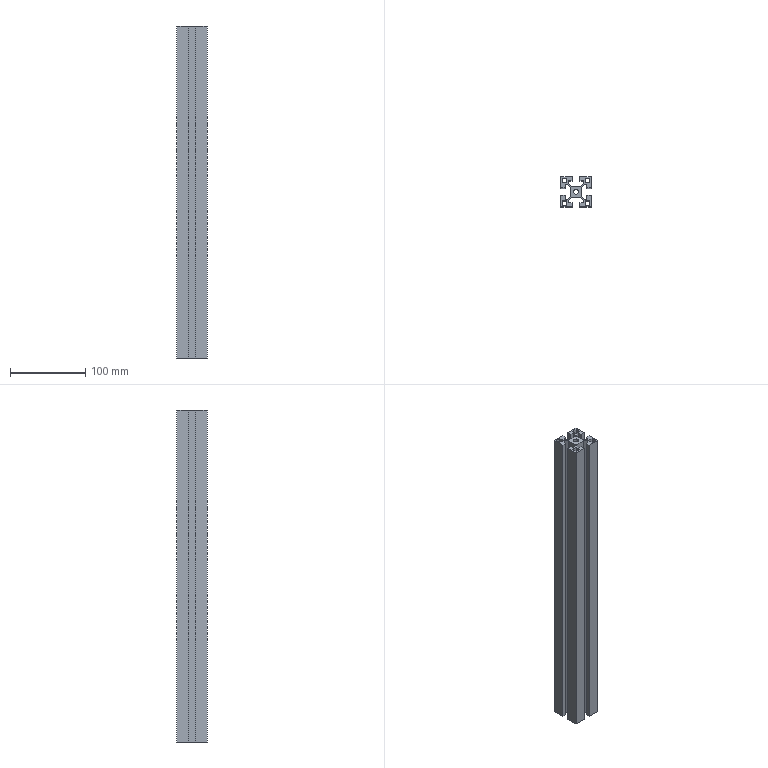Part | STEP file | 4040-2 | 1 solid | 64 faces | box 40 x 40 x 440 mm | volume 309621 mm3 | plane 62 | cylinder 2 | commonest cylinder face diameters 6.8 x2